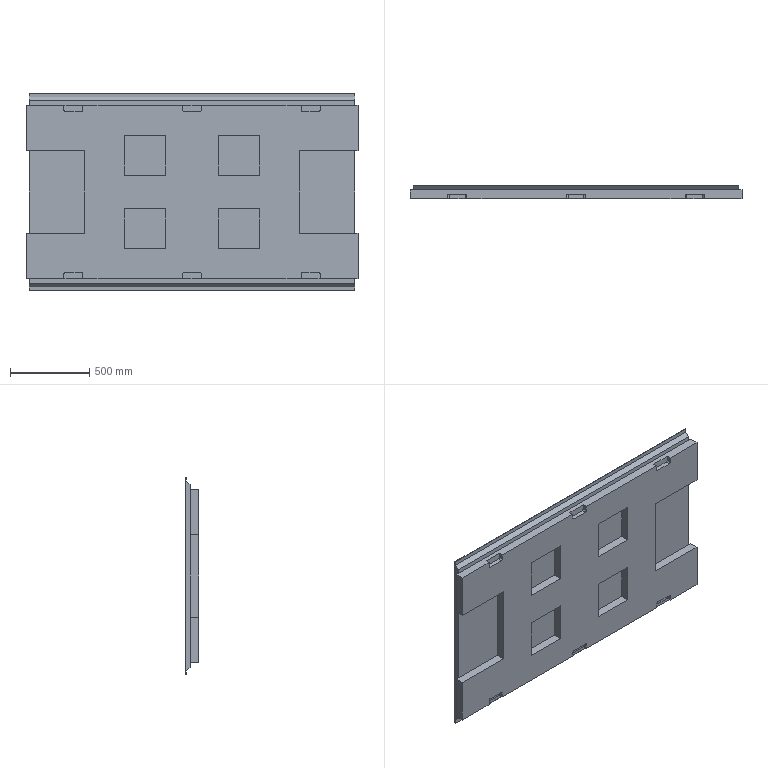Part | SolidWorks | features ICE 3, BaseBody 1 | 2 solids | 267 faces | box 2100 x 85 x 1250 mm | volume 164068651 mm3 | plane 203 | spline 52 | cylinder 12 | commonest cylinder face diameters 20 x12